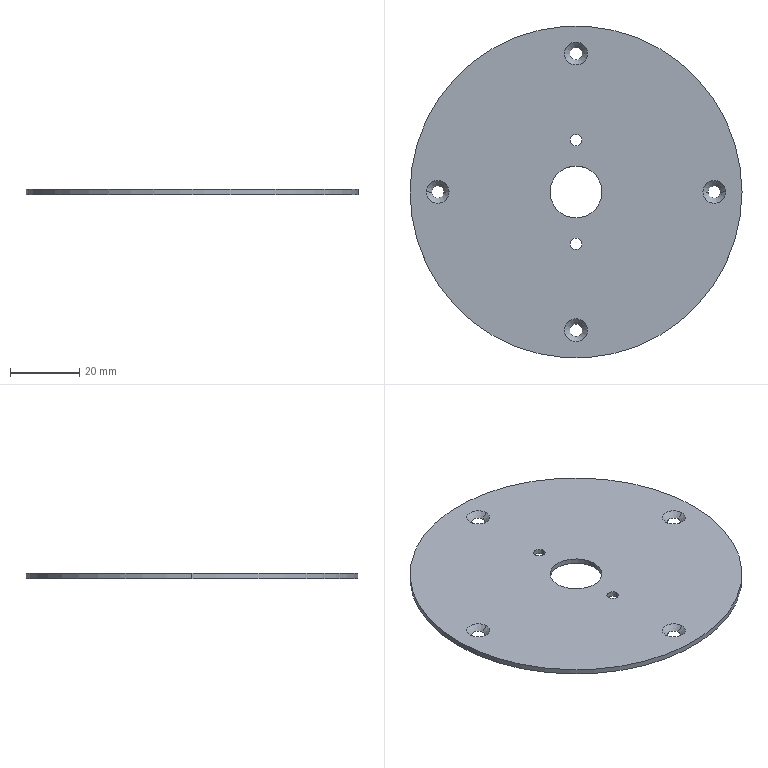Part | STEP file | Twist motor main pulley clamp plate SGN-4-10 | 1 solid | 18 faces | box 96 x 96 x 1.5 mm | volume 10441 mm3 | cylinder 8 | cone 8 | plane 2 | commonest cylinder face diameters 3.3 x4 15 x2 96 x2
STEP:
#1=CARTESIAN_POINT('',(0.,0.,0.));
#2=DIRECTION('',(0.,0.,1.));
#3=DIRECTION('',(1.,0.,0.));
#4=AXIS2_PLACEMENT_3D('',#1,#2,#3);
#5=CARTESIAN_POINT('',(1.65,15.,-1.5));
#6=VERTEX_POINT('',#5);
#7=CARTESIAN_POINT('',(1.65,15.,0.));
#8=VERTEX_POINT('',#7);
#9=CARTESIAN_POINT('',(1.65,15.,0.));
#10=DIRECTION('',(0.,0.,1.));
#11=VECTOR('',#10,1.);
#12=LINE('',#9,#11);
#13=CARTESIAN_POINT('',(0.,15.,0.));
#14=DIRECTION('',(0.,0.,1.));
#15=DIRECTION('',(1.,0.,0.));
#16=AXIS2_PLACEMENT_3D('',#13,#14,#15);
#17=CYLINDRICAL_SURFACE('',#16,1.65);
#18=CARTESIAN_POINT('',(6.283,0.));
#19=DIRECTION('',(0.,1.));
#20=VECTOR('',#19,1.);
#21=LINE('',#18,#20);
#22=(GEOMETRIC_REPRESENTATION_CONTEXT(2)PARAMETRIC_REPRESENTATION_CONTEXT()REPRESENTATION_CONTEXT('',''));
#23=DEFINITIONAL_REPRESENTATION('',(#21),#22);
#24=PCURVE('',#17,#23);
#25=CARTESIAN_POINT('',(0.,15.,0.));
#26=DIRECTION('',(0.,0.,1.));
#27=DIRECTION('',(1.,0.,0.));
#28=AXIS2_PLACEMENT_3D('',#25,#26,#27);
#29=CYLINDRICAL_SURFACE('',#28,1.65);
#30=CARTESIAN_POINT('',(0.,0.));
#31=DIRECTION('',(0.,1.));
#32=VECTOR('',#31,1.);
#33=LINE('',#30,#32);
#34=(GEOMETRIC_REPRESENTATION_CONTEXT(2)PARAMETRIC_REPRESENTATION_CONTEXT()REPRESENTATION_CONTEXT('',''));
#35=DEFINITIONAL_REPRESENTATION('',(#33),#34);
#36=PCURVE('',#29,#35);
#37=SURFACE_CURVE('',#12,(#24,#36),.PCURVE_S1.);
#38=EDGE_CURVE('',#6,#8,#37,.T.);
#39=ORIENTED_EDGE('',*,*,#38,.T.);
#40=CARTESIAN_POINT('',(-1.65,15.,0.));
#41=VERTEX_POINT('',#40);
#42=CARTESIAN_POINT('',(0.,15.,0.));
#43=DIRECTION('',(0.,0.,1.));
#44=DIRECTION('',(1.,0.,0.));
#45=AXIS2_PLACEMENT_3D('',#42,#43,#44);
#46=CIRCLE('',#45,1.65);
#47=CARTESIAN_POINT('',(0.,0.));
#48=DIRECTION('',(1.,0.));
#49=VECTOR('',#48,1.);
#50=LINE('',#47,#49);
#51=(GEOMETRIC_REPRESENTATION_CONTEXT(2)PARAMETRIC_REPRESENTATION_CONTEXT()REPRESENTATION_CONTEXT('',''));
#52=DEFINITIONAL_REPRESENTATION('',(#50),#51);
#53=PCURVE('',#17,#52);
#54=CARTESIAN_POINT('',(0.,0.,0.));
#55=DIRECTION('',(0.,0.,1.));
#56=DIRECTION('',(1.,0.,0.));
#57=AXIS2_PLACEMENT_3D('',#54,#55,#56);
#58=PLANE('',#57);
#59=CARTESIAN_POINT('',(0.,15.));
#60=DIRECTION('',(1.,0.));
#61=AXIS2_PLACEMENT_2D('',#59,#60);
#62=CIRCLE('',#61,1.65);
#63=(GEOMETRIC_REPRESENTATION_CONTEXT(2)PARAMETRIC_REPRESENTATION_CONTEXT()REPRESENTATION_CONTEXT('',''));
#64=DEFINITIONAL_REPRESENTATION('',(#62),#63);
#65=PCURVE('',#58,#64);
#66=SURFACE_CURVE('',#46,(#53,#65),.PCURVE_S1.);
#67=EDGE_CURVE('',#41,#8,#66,.T.);
#68=ORIENTED_EDGE('',*,*,#67,.F.);
#69=CARTESIAN_POINT('',(-1.65,15.,-1.5));
#70=VERTEX_POINT('',#69);
#71=CARTESIAN_POINT('',(-1.65,15.,0.));
#72=DIRECTION('',(0.,0.,1.));
#73=VECTOR('',#72,1.);
#74=LINE('',#71,#73);
#75=CARTESIAN_POINT('',(3.142,0.));
#76=DIRECTION('',(0.,1.));
#77=VECTOR('',#76,1.);
#78=LINE('',#75,#77);
#79=(GEOMETRIC_REPRESENTATION_CONTEXT(2)PARAMETRIC_REPRESENTATION_CONTEXT()REPRESENTATION_CONTEXT('',''));
#80=DEFINITIONAL_REPRESENTATION('',(#78),#79);
#81=PCURVE('',#17,#80);
#82=CARTESIAN_POINT('',(3.142,0.));
#83=DIRECTION('',(0.,1.));
#84=VECTOR('',#83,1.);
#85=LINE('',#82,#84);
#86=(GEOMETRIC_REPRESENTATION_CONTEXT(2)PARAMETRIC_REPRESENTATION_CONTEXT()REPRESENTATION_CONTEXT('',''));
#87=DEFINITIONAL_REPRESENTATION('',(#85),#86);
#88=PCURVE('',#29,#87);
#89=SURFACE_CURVE('',#74,(#81,#88),.PCURVE_S1.);
#90=EDGE_CURVE('',#70,#41,#89,.T.);
#91=ORIENTED_EDGE('',*,*,#90,.F.);
#92=CARTESIAN_POINT('',(0.,15.,-1.5));
#93=DIRECTION('',(0.,0.,1.));
#94=DIRECTION('',(1.,0.,0.));
#95=AXIS2_PLACEMENT_3D('',#92,#93,#94);
#96=CIRCLE('',#95,1.65);
#97=CARTESIAN_POINT('',(0.,-1.5));
#98=DIRECTION('',(1.,0.));
#99=VECTOR('',#98,1.);
#100=LINE('',#97,#99);
#101=(GEOMETRIC_REPRESENTATION_CONTEXT(2)PARAMETRIC_REPRESENTATION_CONTEXT()REPRESENTATION_CONTEXT('',''));
#102=DEFINITIONAL_REPRESENTATION('',(#100),#101);
#103=PCURVE('',#17,#102);
#104=CARTESIAN_POINT('',(0.,0.,-1.5));
#105=DIRECTION('',(0.,0.,1.));
#106=DIRECTION('',(1.,0.,0.));
#107=AXIS2_PLACEMENT_3D('',#104,#105,#106);
#108=PLANE('',#107);
#109=CARTESIAN_POINT('',(0.,15.));
#110=DIRECTION('',(1.,0.));
#111=AXIS2_PLACEMENT_2D('',#109,#110);
#112=CIRCLE('',#111,1.65);
#113=(GEOMETRIC_REPRESENTATION_CONTEXT(2)PARAMETRIC_REPRESENTATION_CONTEXT()REPRESENTATION_CONTEXT('',''));
#114=DEFINITIONAL_REPRESENTATION('',(#112),#113);
#115=PCURVE('',#108,#114);
#116=SURFACE_CURVE('',#96,(#103,#115),.PCURVE_S1.);
#117=EDGE_CURVE('',#70,#6,#116,.T.);
#118=ORIENTED_EDGE('',*,*,#117,.T.);
#119=EDGE_LOOP('',(#39,#68,#91,#118));
#120=FACE_BOUND('',#119,.F.);
#121=ADVANCED_FACE('',(#120),#17,.F.);
#122=CARTESIAN_POINT('',(1.65,-15.,-1.5));
#123=VERTEX_POINT('',#122);
#124=CARTESIAN_POINT('',(1.65,-15.,0.));
#125=VERTEX_POINT('',#124);
#126=CARTESIAN_POINT('',(1.65,-15.,0.));
#127=DIRECTION('',(0.,0.,1.));
#128=VECTOR('',#127,1.);
#129=LINE('',#126,#128);
#130=CARTESIAN_POINT('',(0.,-15.,0.));
#131=DIRECTION('',(0.,0.,1.));
#132=DIRECTION('',(1.,0.,0.));
#133=AXIS2_PLACEMENT_3D('',#130,#131,#132);
#134=CYLINDRICAL_SURFACE('',#133,1.65);
#135=CARTESIAN_POINT('',(6.283,0.));
#136=DIRECTION('',(0.,1.));
#137=VECTOR('',#136,1.);
#138=LINE('',#135,#137);
#139=(GEOMETRIC_REPRESENTATION_CONTEXT(2)PARAMETRIC_REPRESENTATION_CONTEXT()REPRESENTATION_CONTEXT('',''));
#140=DEFINITIONAL_REPRESENTATION('',(#138),#139);
#141=PCURVE('',#134,#140);
#142=CARTESIAN_POINT('',(0.,-15.,0.));
#143=DIRECTION('',(0.,0.,1.));
#144=DIRECTION('',(1.,0.,0.));
#145=AXIS2_PLACEMENT_3D('',#142,#143,#144);
#146=CYLINDRICAL_SURFACE('',#145,1.65);
#147=CARTESIAN_POINT('',(0.,0.));
#148=DIRECTION('',(0.,1.));
#149=VECTOR('',#148,1.);
#150=LINE('',#147,#149);
#151=(GEOMETRIC_REPRESENTATION_CONTEXT(2)PARAMETRIC_REPRESENTATION_CONTEXT()REPRESENTATION_CONTEXT('',''));
#152=DEFINITIONAL_REPRESENTATION('',(#150),#151);
#153=PCURVE('',#146,#152);
#154=SURFACE_CURVE('',#129,(#141,#153),.PCURVE_S1.);
#155=EDGE_CURVE('',#123,#125,#154,.T.);
#156=ORIENTED_EDGE('',*,*,#155,.T.);
#157=CARTESIAN_POINT('',(-1.65,-15.,0.));
#158=VERTEX_POINT('',#157);
#159=CARTESIAN_POINT('',(0.,-15.,0.));
#160=DIRECTION('',(0.,0.,1.));
#161=DIRECTION('',(1.,0.,0.));
#162=AXIS2_PLACEMENT_3D('',#159,#160,#161);
#163=CIRCLE('',#162,1.65);
#164=CARTESIAN_POINT('',(0.,0.));
#165=DIRECTION('',(1.,0.));
#166=VECTOR('',#165,1.);
#167=LINE('',#164,#166);
#168=(GEOMETRIC_REPRESENTATION_CONTEXT(2)PARAMETRIC_REPRESENTATION_CONTEXT()REPRESENTATION_CONTEXT('',''));
#169=DEFINITIONAL_REPRESENTATION('',(#167),#168);
#170=PCURVE('',#134,#169);
#171=CARTESIAN_POINT('',(0.,-15.));
#172=DIRECTION('',(1.,0.));
#173=AXIS2_PLACEMENT_2D('',#171,#172);
#174=CIRCLE('',#173,1.65);
#175=(GEOMETRIC_REPRESENTATION_CONTEXT(2)PARAMETRIC_REPRESENTATION_CONTEXT()REPRESENTATION_CONTEXT('',''));
#176=DEFINITIONAL_REPRESENTATION('',(#174),#175);
#177=PCURVE('',#58,#176);
#178=SURFACE_CURVE('',#163,(#170,#177),.PCURVE_S1.);
#179=EDGE_CURVE('',#158,#125,#178,.T.);
#180=ORIENTED_EDGE('',*,*,#179,.F.);
#181=CARTESIAN_POINT('',(-1.65,-15.,-1.5));
#182=VERTEX_POINT('',#181);
#183=CARTESIAN_POINT('',(-1.65,-15.,0.));
#184=DIRECTION('',(0.,0.,1.));
#185=VECTOR('',#184,1.);
#186=LINE('',#183,#185);
#187=CARTESIAN_POINT('',(3.142,0.));
#188=DIRECTION('',(0.,1.));
#189=VECTOR('',#188,1.);
#190=LINE('',#187,#189);
#191=(GEOMETRIC_REPRESENTATION_CONTEXT(2)PARAMETRIC_REPRESENTATION_CONTEXT()REPRESENTATION_CONTEXT('',''));
#192=DEFINITIONAL_REPRESENTATION('',(#190),#191);
#193=PCURVE('',#134,#192);
#194=CARTESIAN_POINT('',(3.142,0.));
#195=DIRECTION('',(0.,1.));
#196=VECTOR('',#195,1.);
#197=LINE('',#194,#196);
#198=(GEOMETRIC_REPRESENTATION_CONTEXT(2)PARAMETRIC_REPRESENTATION_CONTEXT()REPRESENTATION_CONTEXT('',''));
#199=DEFINITIONAL_REPRESENTATION('',(#197),#198);
#200=PCURVE('',#146,#199);
#201=SURFACE_CURVE('',#186,(#193,#200),.PCURVE_S1.);
#202=EDGE_CURVE('',#182,#158,#201,.T.);
#203=ORIENTED_EDGE('',*,*,#202,.F.);
#204=CARTESIAN_POINT('',(0.,-15.,-1.5));
#205=DIRECTION('',(0.,0.,1.));
#206=DIRECTION('',(1.,0.,0.));
#207=AXIS2_PLACEMENT_3D('',#204,#205,#206);
#208=CIRCLE('',#207,1.65);
#209=CARTESIAN_POINT('',(0.,-1.5));
#210=DIRECTION('',(1.,0.));
#211=VECTOR('',#210,1.);
#212=LINE('',#209,#211);
#213=(GEOMETRIC_REPRESENTATION_CONTEXT(2)PARAMETRIC_REPRESENTATION_CONTEXT()REPRESENTATION_CONTEXT('',''));
#214=DEFINITIONAL_REPRESENTATION('',(#212),#213);
#215=PCURVE('',#134,#214);
#216=CARTESIAN_POINT('',(0.,-15.));
#217=DIRECTION('',(1.,0.));
#218=AXIS2_PLACEMENT_2D('',#216,#217);
#219=CIRCLE('',#218,1.65);
#220=(GEOMETRIC_REPRESENTATION_CONTEXT(2)PARAMETRIC_REPRESENTATION_CONTEXT()REPRESENTATION_CONTEXT('',''));
#221=DEFINITIONAL_REPRESENTATION('',(#219),#220);
#222=PCURVE('',#108,#221);
#223=SURFACE_CURVE('',#208,(#215,#222),.PCURVE_S1.);
#224=EDGE_CURVE('',#182,#123,#223,.T.);
#225=ORIENTED_EDGE('',*,*,#224,.T.);
#226=EDGE_LOOP('',(#156,#180,#203,#225));
#227=FACE_BOUND('',#226,.F.);
#228=ADVANCED_FACE('',(#227),#134,.F.);
#229=CARTESIAN_POINT('',(7.5,0.,-1.5));
#230=VERTEX_POINT('',#229);
#231=CARTESIAN_POINT('',(7.5,0.,0.));
#232=VERTEX_POINT('',#231);
#233=CARTESIAN_POINT('',(7.5,0.,-10.));
#234=DIRECTION('',(0.,0.,1.));
#235=VECTOR('',#234,1.);
#236=LINE('',#233,#235);
#237=CARTESIAN_POINT('',(0.,0.,-10.));
#238=DIRECTION('',(0.,0.,1.));
#239=DIRECTION('',(1.,0.,0.));
#240=AXIS2_PLACEMENT_3D('',#237,#238,#239);
#241=CYLINDRICAL_SURFACE('',#240,7.5);
#242=CARTESIAN_POINT('',(6.283,0.));
#243=DIRECTION('',(0.,1.));
#244=VECTOR('',#243,1.);
#245=LINE('',#242,#244);
#246=(GEOMETRIC_REPRESENTATION_CONTEXT(2)PARAMETRIC_REPRESENTATION_CONTEXT()REPRESENTATION_CONTEXT('',''));
#247=DEFINITIONAL_REPRESENTATION('',(#245),#246);
#248=PCURVE('',#241,#247);
#249=CARTESIAN_POINT('',(0.,0.,-10.));
#250=DIRECTION('',(0.,0.,1.));
#251=DIRECTION('',(1.,0.,0.));
#252=AXIS2_PLACEMENT_3D('',#249,#250,#251);
#253=CYLINDRICAL_SURFACE('',#252,7.5);
#254=CARTESIAN_POINT('',(0.,0.));
#255=DIRECTION('',(0.,1.));
#256=VECTOR('',#255,1.);
#257=LINE('',#254,#256);
#258=(GEOMETRIC_REPRESENTATION_CONTEXT(2)PARAMETRIC_REPRESENTATION_CONTEXT()REPRESENTATION_CONTEXT('',''));
#259=DEFINITIONAL_REPRESENTATION('',(#257),#258);
#260=PCURVE('',#253,#259);
#261=SURFACE_CURVE('',#236,(#248,#260),.PCURVE_S1.);
#262=EDGE_CURVE('',#230,#232,#261,.T.);
#263=ORIENTED_EDGE('',*,*,#262,.T.);
#264=CARTESIAN_POINT('',(-7.5,0.,0.));
#265=VERTEX_POINT('',#264);
#266=CARTESIAN_POINT('',(0.,0.,0.));
#267=DIRECTION('',(0.,0.,1.));
#268=DIRECTION('',(1.,0.,0.));
#269=AXIS2_PLACEMENT_3D('',#266,#267,#268);
#270=CIRCLE('',#269,7.5);
#271=CARTESIAN_POINT('',(0.,10.));
#272=DIRECTION('',(1.,0.));
#273=VECTOR('',#272,1.);
#274=LINE('',#271,#273);
#275=(GEOMETRIC_REPRESENTATION_CONTEXT(2)PARAMETRIC_REPRESENTATION_CONTEXT()REPRESENTATION_CONTEXT('',''));
#276=DEFINITIONAL_REPRESENTATION('',(#274),#275);
#277=PCURVE('',#241,#276);
#278=CARTESIAN_POINT('',(0.,0.));
#279=DIRECTION('',(1.,0.));
#280=AXIS2_PLACEMENT_2D('',#278,#279);
#281=CIRCLE('',#280,7.5);
#282=(GEOMETRIC_REPRESENTATION_CONTEXT(2)PARAMETRIC_REPRESENTATION_CONTEXT()REPRESENTATION_CONTEXT('',''));
#283=DEFINITIONAL_REPRESENTATION('',(#281),#282);
#284=PCURVE('',#58,#283);
#285=SURFACE_CURVE('',#270,(#277,#284),.PCURVE_S1.);
#286=EDGE_CURVE('',#265,#232,#285,.T.);
#287=ORIENTED_EDGE('',*,*,#286,.F.);
#288=CARTESIAN_POINT('',(-7.5,0.,-1.5));
#289=VERTEX_POINT('',#288);
#290=CARTESIAN_POINT('',(-7.5,0.,-10.));
#291=DIRECTION('',(0.,0.,1.));
#292=VECTOR('',#291,1.);
#293=LINE('',#290,#292);
#294=CARTESIAN_POINT('',(3.142,0.));
#295=DIRECTION('',(0.,1.));
#296=VECTOR('',#295,1.);
#297=LINE('',#294,#296);
#298=(GEOMETRIC_REPRESENTATION_CONTEXT(2)PARAMETRIC_REPRESENTATION_CONTEXT()REPRESENTATION_CONTEXT('',''));
#299=DEFINITIONAL_REPRESENTATION('',(#297),#298);
#300=PCURVE('',#241,#299);
#301=CARTESIAN_POINT('',(3.142,0.));
#302=DIRECTION('',(0.,1.));
#303=VECTOR('',#302,1.);
#304=LINE('',#301,#303);
#305=(GEOMETRIC_REPRESENTATION_CONTEXT(2)PARAMETRIC_REPRESENTATION_CONTEXT()REPRESENTATION_CONTEXT('',''));
#306=DEFINITIONAL_REPRESENTATION('',(#304),#305);
#307=PCURVE('',#253,#306);
#308=SURFACE_CURVE('',#293,(#300,#307),.PCURVE_S1.);
#309=EDGE_CURVE('',#289,#265,#308,.T.);
#310=ORIENTED_EDGE('',*,*,#309,.F.);
#311=CARTESIAN_POINT('',(0.,0.,-1.5));
#312=DIRECTION('',(0.,0.,1.));
#313=DIRECTION('',(1.,0.,0.));
#314=AXIS2_PLACEMENT_3D('',#311,#312,#313);
#315=CIRCLE('',#314,7.5);
#316=CARTESIAN_POINT('',(0.,8.5));
#317=DIRECTION('',(1.,0.));
#318=VECTOR('',#317,1.);
#319=LINE('',#316,#318);
#320=(GEOMETRIC_REPRESENTATION_CONTEXT(2)PARAMETRIC_REPRESENTATION_CONTEXT()REPRESENTATION_CONTEXT('',''));
#321=DEFINITIONAL_REPRESENTATION('',(#319),#320);
#322=PCURVE('',#241,#321);
#323=CARTESIAN_POINT('',(0.,0.));
#324=DIRECTION('',(1.,0.));
#325=AXIS2_PLACEMENT_2D('',#323,#324);
#326=CIRCLE('',#325,7.5);
#327=(GEOMETRIC_REPRESENTATION_CONTEXT(2)PARAMETRIC_REPRESENTATION_CONTEXT()REPRESENTATION_CONTEXT('',''));
#328=DEFINITIONAL_REPRESENTATION('',(#326),#327);
#329=PCURVE('',#108,#328);
#330=SURFACE_CURVE('',#315,(#322,#329),.PCURVE_S1.);
#331=EDGE_CURVE('',#289,#230,#330,.T.);
#332=ORIENTED_EDGE('',*,*,#331,.T.);
#333=EDGE_LOOP('',(#263,#287,#310,#332));
#334=FACE_BOUND('',#333,.F.);
#335=ADVANCED_FACE('',(#334),#241,.F.);
#336=CARTESIAN_POINT('',(1.8,40.,-1.5));
#337=VERTEX_POINT('',#336);
#338=CARTESIAN_POINT('',(3.3,40.,0.));
#339=VERTEX_POINT('',#338);
#340=CARTESIAN_POINT('',(3.3,40.,0.));
#341=DIRECTION('',(0.7071,0.,0.7071));
#342=VECTOR('',#341,1.);
#343=LINE('',#340,#342);
#344=CARTESIAN_POINT('',(0.,40.,0.));
#345=DIRECTION('',(0.,0.,1.));
#346=DIRECTION('',(1.,0.,0.));
#347=AXIS2_PLACEMENT_3D('',#344,#345,#346);
#348=CONICAL_SURFACE('',#347,3.3,0.7854);
#349=CARTESIAN_POINT('',(6.283,0.));
#350=DIRECTION('',(0.,1.));
#351=VECTOR('',#350,1.);
#352=LINE('',#349,#351);
#353=(GEOMETRIC_REPRESENTATION_CONTEXT(2)PARAMETRIC_REPRESENTATION_CONTEXT()REPRESENTATION_CONTEXT('',''));
#354=DEFINITIONAL_REPRESENTATION('',(#352),#353);
#355=PCURVE('',#348,#354);
#356=CARTESIAN_POINT('',(0.,40.,0.));
#357=DIRECTION('',(0.,0.,1.));
#358=DIRECTION('',(1.,0.,0.));
#359=AXIS2_PLACEMENT_3D('',#356,#357,#358);
#360=CONICAL_SURFACE('',#359,3.3,0.7854);
#361=CARTESIAN_POINT('',(0.,0.));
#362=DIRECTION('',(0.,1.));
#363=VECTOR('',#362,1.);
#364=LINE('',#361,#363);
#365=(GEOMETRIC_REPRESENTATION_CONTEXT(2)PARAMETRIC_REPRESENTATION_CONTEXT()REPRESENTATION_CONTEXT('',''));
#366=DEFINITIONAL_REPRESENTATION('',(#364),#365);
#367=PCURVE('',#360,#366);
#368=SURFACE_CURVE('',#343,(#355,#367),.PCURVE_S1.);
#369=EDGE_CURVE('',#337,#339,#368,.T.);
#370=ORIENTED_EDGE('',*,*,#369,.T.);
#371=CARTESIAN_POINT('',(-3.3,40.,0.));
#372=VERTEX_POINT('',#371);
#373=CARTESIAN_POINT('',(0.,40.,0.));
#374=DIRECTION('',(0.,0.,1.));
#375=DIRECTION('',(1.,0.,0.));
#376=AXIS2_PLACEMENT_3D('',#373,#374,#375);
#377=CIRCLE('',#376,3.3);
#378=CARTESIAN_POINT('',(0.,0.));
#379=DIRECTION('',(1.,0.));
#380=VECTOR('',#379,1.);
#381=LINE('',#378,#380);
#382=(GEOMETRIC_REPRESENTATION_CONTEXT(2)PARAMETRIC_REPRESENTATION_CONTEXT()REPRESENTATION_CONTEXT('',''));
#383=DEFINITIONAL_REPRESENTATION('',(#381),#382);
#384=PCURVE('',#348,#383);
#385=CARTESIAN_POINT('',(0.,40.));
#386=DIRECTION('',(1.,0.));
#387=AXIS2_PLACEMENT_2D('',#385,#386);
#388=CIRCLE('',#387,3.3);
#389=(GEOMETRIC_REPRESENTATION_CONTEXT(2)PARAMETRIC_REPRESENTATION_CONTEXT()REPRESENTATION_CONTEXT('',''));
#390=DEFINITIONAL_REPRESENTATION('',(#388),#389);
#391=PCURVE('',#58,#390);
#392=SURFACE_CURVE('',#377,(#384,#391),.PCURVE_S1.);
#393=EDGE_CURVE('',#372,#339,#392,.T.);
#394=ORIENTED_EDGE('',*,*,#393,.F.);
#395=CARTESIAN_POINT('',(-1.8,40.,-1.5));
#396=VERTEX_POINT('',#395);
#397=CARTESIAN_POINT('',(-3.3,40.,0.));
#398=DIRECTION('',(-0.7071,0.,0.7071));
#399=VECTOR('',#398,1.);
#400=LINE('',#397,#399);
#401=CARTESIAN_POINT('',(3.142,0.));
#402=DIRECTION('',(0.,1.));
#403=VECTOR('',#402,1.);
#404=LINE('',#401,#403);
#405=(GEOMETRIC_REPRESENTATION_CONTEXT(2)PARAMETRIC_REPRESENTATION_CONTEXT()REPRESENTATION_CONTEXT('',''));
#406=DEFINITIONAL_REPRESENTATION('',(#404),#405);
#407=PCURVE('',#348,#406);
#408=CARTESIAN_POINT('',(3.142,0.));
#409=DIRECTION('',(0.,1.));
#410=VECTOR('',#409,1.);
#411=LINE('',#408,#410);
#412=(GEOMETRIC_REPRESENTATION_CONTEXT(2)PARAMETRIC_REPRESENTATION_CONTEXT()REPRESENTATION_CONTEXT('',''));
#413=DEFINITIONAL_REPRESENTATION('',(#411),#412);
#414=PCURVE('',#360,#413);
#415=SURFACE_CURVE('',#400,(#407,#414),.PCURVE_S1.);
#416=EDGE_CURVE('',#396,#372,#415,.T.);
#417=ORIENTED_EDGE('',*,*,#416,.F.);
#418=CARTESIAN_POINT('',(0.,40.,-1.5));
#419=DIRECTION('',(0.,0.,1.));
#420=DIRECTION('',(1.,0.,0.));
#421=AXIS2_PLACEMENT_3D('',#418,#419,#420);
#422=CIRCLE('',#421,1.8);
#423=CARTESIAN_POINT('',(0.,-1.5));
#424=DIRECTION('',(1.,0.));
#425=VECTOR('',#424,1.);
#426=LINE('',#423,#425);
#427=(GEOMETRIC_REPRESENTATION_CONTEXT(2)PARAMETRIC_REPRESENTATION_CONTEXT()REPRESENTATION_CONTEXT('',''));
#428=DEFINITIONAL_REPRESENTATION('',(#426),#427);
#429=PCURVE('',#348,#428);
#430=CARTESIAN_POINT('',(0.,40.));
#431=DIRECTION('',(1.,0.));
#432=AXIS2_PLACEMENT_2D('',#430,#431);
#433=CIRCLE('',#432,1.8);
#434=(GEOMETRIC_REPRESENTATION_CONTEXT(2)PARAMETRIC_REPRESENTATION_CONTEXT()REPRESENTATION_CONTEXT('',''));
#435=DEFINITIONAL_REPRESENTATION('',(#433),#434);
#436=PCURVE('',#108,#435);
#437=SURFACE_CURVE('',#422,(#429,#436),.PCURVE_S1.);
#438=EDGE_CURVE('',#396,#337,#437,.T.);
#439=ORIENTED_EDGE('',*,*,#438,.T.);
#440=EDGE_LOOP('',(#370,#394,#417,#439));
#441=FACE_BOUND('',#440,.F.);
#442=ADVANCED_FACE('',(#441),#348,.F.);
#443=CARTESIAN_POINT('',(41.8,0.,-1.5));
#444=VERTEX_POINT('',#443);
#445=CARTESIAN_POINT('',(43.3,0.,0.));
#446=VERTEX_POINT('',#445);
#447=CARTESIAN_POINT('',(43.3,0.,0.));
#448=DIRECTION('',(0.7071,0.,0.7071));
#449=VECTOR('',#448,1.);
#450=LINE('',#447,#449);
#451=CARTESIAN_POINT('',(40.,0.,0.));
#452=DIRECTION('',(0.,0.,1.));
#453=DIRECTION('',(1.,0.,0.));
#454=AXIS2_PLACEMENT_3D('',#451,#452,#453);
#455=CONICAL_SURFACE('',#454,3.3,0.7854);
#456=CARTESIAN_POINT('',(6.283,0.));
#457=DIRECTION('',(0.,1.));
#458=VECTOR('',#457,1.);
#459=LINE('',#456,#458);
#460=(GEOMETRIC_REPRESENTATION_CONTEXT(2)PARAMETRIC_REPRESENTATION_CONTEXT()REPRESENTATION_CONTEXT('',''));
#461=DEFINITIONAL_REPRESENTATION('',(#459),#460);
#462=PCURVE('',#455,#461);
#463=CARTESIAN_POINT('',(40.,0.,0.));
#464=DIRECTION('',(0.,0.,1.));
#465=DIRECTION('',(1.,0.,0.));
#466=AXIS2_PLACEMENT_3D('',#463,#464,#465);
#467=CONICAL_SURFACE('',#466,3.3,0.7854);
#468=CARTESIAN_POINT('',(0.,0.));
#469=DIRECTION('',(0.,1.));
#470=VECTOR('',#469,1.);
#471=LINE('',#468,#470);
#472=(GEOMETRIC_REPRESENTATION_CONTEXT(2)PARAMETRIC_REPRESENTATION_CONTEXT()REPRESENTATION_CONTEXT('',''));
#473=DEFINITIONAL_REPRESENTATION('',(#471),#472);
#474=PCURVE('',#467,#473);
#475=SURFACE_CURVE('',#450,(#462,#474),.PCURVE_S1.);
#476=EDGE_CURVE('',#444,#446,#475,.T.);
#477=ORIENTED_EDGE('',*,*,#476,.T.);
#478=CARTESIAN_POINT('',(36.7,0.,0.));
#479=VERTEX_POINT('',#478);
#480=CARTESIAN_POINT('',(40.,0.,0.));
#481=DIRECTION('',(0.,0.,1.));
#482=DIRECTION('',(1.,0.,0.));
#483=AXIS2_PLACEMENT_3D('',#480,#481,#482);
#484=CIRCLE('',#483,3.3);
#485=CARTESIAN_POINT('',(0.,0.));
#486=DIRECTION('',(1.,0.));
#487=VECTOR('',#486,1.);
#488=LINE('',#485,#487);
#489=(GEOMETRIC_REPRESENTATION_CONTEXT(2)PARAMETRIC_REPRESENTATION_CONTEXT()REPRESENTATION_CONTEXT('',''));
#490=DEFINITIONAL_REPRESENTATION('',(#488),#489);
#491=PCURVE('',#455,#490);
#492=CARTESIAN_POINT('',(40.,0.));
#493=DIRECTION('',(1.,0.));
#494=AXIS2_PLACEMENT_2D('',#492,#493);
#495=CIRCLE('',#494,3.3);
#496=(GEOMETRIC_REPRESENTATION_CONTEXT(2)PARAMETRIC_REPRESENTATION_CONTEXT()REPRESENTATION_CONTEXT('',''));
#497=DEFINITIONAL_REPRESENTATION('',(#495),#496);
#498=PCURVE('',#58,#497);
#499=SURFACE_CURVE('',#484,(#491,#498),.PCURVE_S1.);
#500=EDGE_CURVE('',#479,#446,#499,.T.);
#501=ORIENTED_EDGE('',*,*,#500,.F.);
#502=CARTESIAN_POINT('',(38.2,0.,-1.5));
#503=VERTEX_POINT('',#502);
#504=CARTESIAN_POINT('',(36.7,0.,0.));
#505=DIRECTION('',(-0.7071,0.,0.7071));
#506=VECTOR('',#505,1.);
#507=LINE('',#504,#506);
#508=CARTESIAN_POINT('',(3.142,0.));
#509=DIRECTION('',(0.,1.));
#510=VECTOR('',#509,1.);
#511=LINE('',#508,#510);
#512=(GEOMETRIC_REPRESENTATION_CONTEXT(2)PARAMETRIC_REPRESENTATION_CONTEXT()REPRESENTATION_CONTEXT('',''));
#513=DEFINITIONAL_REPRESENTATION('',(#511),#512);
#514=PCURVE('',#455,#513);
#515=CARTESIAN_POINT('',(3.142,0.));
#516=DIRECTION('',(0.,1.));
#517=VECTOR('',#516,1.);
#518=LINE('',#515,#517);
#519=(GEOMETRIC_REPRESENTATION_CONTEXT(2)PARAMETRIC_REPRESENTATION_CONTEXT()REPRESENTATION_CONTEXT('',''));
#520=DEFINITIONAL_REPRESENTATION('',(#518),#519);
#521=PCURVE('',#467,#520);
#522=SURFACE_CURVE('',#507,(#514,#521),.PCURVE_S1.);
#523=EDGE_CURVE('',#503,#479,#522,.T.);
#524=ORIENTED_EDGE('',*,*,#523,.F.);
#525=CARTESIAN_POINT('',(40.,0.,-1.5));
#526=DIRECTION('',(0.,0.,1.));
#527=DIRECTION('',(1.,0.,0.));
#528=AXIS2_PLACEMENT_3D('',#525,#526,#527);
#529=CIRCLE('',#528,1.8);
#530=CARTESIAN_POINT('',(0.,-1.5));
#531=DIRECTION('',(1.,0.));
#532=VECTOR('',#531,1.);
#533=LINE('',#530,#532);
#534=(GEOMETRIC_REPRESENTATION_CONTEXT(2)PARAMETRIC_REPRESENTATION_CONTEXT()REPRESENTATION_CONTEXT('',''));
#535=DEFINITIONAL_REPRESENTATION('',(#533),#534);
#536=PCURVE('',#455,#535);
#537=CARTESIAN_POINT('',(40.,0.));
#538=DIRECTION('',(1.,0.));
#539=AXIS2_PLACEMENT_2D('',#537,#538);
#540=CIRCLE('',#539,1.8);
#541=(GEOMETRIC_REPRESENTATION_CONTEXT(2)PARAMETRIC_REPRESENTATION_CONTEXT()REPRESENTATION_CONTEXT('',''));
#542=DEFINITIONAL_REPRESENTATION('',(#540),#541);
#543=PCURVE('',#108,#542);
#544=SURFACE_CURVE('',#529,(#536,#543),.PCURVE_S1.);
#545=EDGE_CURVE('',#503,#444,#544,.T.);
#546=ORIENTED_EDGE('',*,*,#545,.T.);
#547=EDGE_LOOP('',(#477,#501,#524,#546));
#548=FACE_BOUND('',#547,.F.);
#549=ADVANCED_FACE('',(#548),#455,.F.);
#550=CARTESIAN_POINT('',(1.8,-40.,-1.5));
#551=VERTEX_POINT('',#550);
#552=CARTESIAN_POINT('',(3.3,-40.,0.));
#553=VERTEX_POINT('',#552);
#554=CARTESIAN_POINT('',(3.3,-40.,0.));
#555=DIRECTION('',(0.7071,0.,0.7071));
#556=VECTOR('',#555,1.);
#557=LINE('',#554,#556);
#558=CARTESIAN_POINT('',(0.,-40.,0.));
#559=DIRECTION('',(0.,0.,1.));
#560=DIRECTION('',(1.,0.,0.));
#561=AXIS2_PLACEMENT_3D('',#558,#559,#560);
#562=CONICAL_SURFACE('',#561,3.3,0.7854);
#563=CARTESIAN_POINT('',(6.283,0.));
#564=DIRECTION('',(0.,1.));
#565=VECTOR('',#564,1.);
#566=LINE('',#563,#565);
#567=(GEOMETRIC_REPRESENTATION_CONTEXT(2)PARAMETRIC_REPRESENTATION_CONTEXT()REPRESENTATION_CONTEXT('',''));
#568=DEFINITIONAL_REPRESENTATION('',(#566),#567);
#569=PCURVE('',#562,#568);
#570=CARTESIAN_POINT('',(0.,-40.,0.));
#571=DIRECTION('',(0.,0.,1.));
#572=DIRECTION('',(1.,0.,0.));
#573=AXIS2_PLACEMENT_3D('',#570,#571,#572);
#574=CONICAL_SURFACE('',#573,3.3,0.7854);
#575=CARTESIAN_POINT('',(0.,0.));
#576=DIRECTION('',(0.,1.));
#577=VECTOR('',#576,1.);
#578=LINE('',#575,#577);
#579=(GEOMETRIC_REPRESENTATION_CONTEXT(2)PARAMETRIC_REPRESENTATION_CONTEXT()REPRESENTATION_CONTEXT('',''));
#580=DEFINITIONAL_REPRESENTATION('',(#578),#579);
#581=PCURVE('',#574,#580);
#582=SURFACE_CURVE('',#557,(#569,#581),.PCURVE_S1.);
#583=EDGE_CURVE('',#551,#553,#582,.T.);
#584=ORIENTED_EDGE('',*,*,#583,.T.);
#585=CARTESIAN_POINT('',(-3.3,-40.,0.));
#586=VERTEX_POINT('',#585);
#587=CARTESIAN_POINT('',(0.,-40.,0.));
#588=DIRECTION('',(0.,0.,1.));
#589=DIRECTION('',(1.,0.,0.));
#590=AXIS2_PLACEMENT_3D('',#587,#588,#589);
#591=CIRCLE('',#590,3.3);
#592=CARTESIAN_POINT('',(0.,0.));
#593=DIRECTION('',(1.,0.));
#594=VECTOR('',#593,1.);
#595=LINE('',#592,#594);
#596=(GEOMETRIC_REPRESENTATION_CONTEXT(2)PARAMETRIC_REPRESENTATION_CONTEXT()REPRESENTATION_CONTEXT('',''));
#597=DEFINITIONAL_REPRESENTATION('',(#595),#596);
#598=PCURVE('',#562,#597);
#599=CARTESIAN_POINT('',(0.,-40.));
#600=DIRECTION('',(1.,0.));
#601=AXIS2_PLACEMENT_2D('',#599,#600);
#602=CIRCLE('',#601,3.3);
#603=(GEOMETRIC_REPRESENTATION_CONTEXT(2)PARAMETRIC_REPRESENTATION_CONTEXT()REPRESENTATION_CONTEXT('',''));
#604=DEFINITIONAL_REPRESENTATION('',(#602),#603);
#605=PCURVE('',#58,#604);
#606=SURFACE_CURVE('',#591,(#598,#605),.PCURVE_S1.);
#607=EDGE_CURVE('',#586,#553,#606,.T.);
#608=ORIENTED_EDGE('',*,*,#607,.F.);
#609=CARTESIAN_POINT('',(-1.8,-40.,-1.5));
#610=VERTEX_POINT('',#609);
#611=CARTESIAN_POINT('',(-3.3,-40.,0.));
#612=DIRECTION('',(-0.7071,0.,0.7071));
#613=VECTOR('',#612,1.);
#614=LINE('',#611,#613);
#615=CARTESIAN_POINT('',(3.142,0.));
#616=DIRECTION('',(0.,1.));
#617=VECTOR('',#616,1.);
#618=LINE('',#615,#617);
#619=(GEOMETRIC_REPRESENTATION_CONTEXT(2)PARAMETRIC_REPRESENTATION_CONTEXT()REPRESENTATION_CONTEXT('',''));
#620=DEFINITIONAL_REPRESENTATION('',(#618),#619);
#621=PCURVE('',#562,#620);
#622=CARTESIAN_POINT('',(3.142,0.));
#623=DIRECTION('',(0.,1.));
#624=VECTOR('',#623,1.);
#625=LINE('',#622,#624);
#626=(GEOMETRIC_REPRESENTATION_CONTEXT(2)PARAMETRIC_REPRESENTATION_CONTEXT()REPRESENTATION_CONTEXT('',''));
#627=DEFINITIONAL_REPRESENTATION('',(#625),#626);
#628=PCURVE('',#574,#627);
#629=SURFACE_CURVE('',#614,(#621,#628),.PCURVE_S1.);
#630=EDGE_CURVE('',#610,#586,#629,.T.);
#631=ORIENTED_EDGE('',*,*,#630,.F.);
#632=CARTESIAN_POINT('',(0.,-40.,-1.5));
#633=DIRECTION('',(0.,0.,1.));
#634=DIRECTION('',(1.,0.,0.));
#635=AXIS2_PLACEMENT_3D('',#632,#633,#634);
#636=CIRCLE('',#635,1.8);
#637=CARTESIAN_POINT('',(0.,-1.5));
#638=DIRECTION('',(1.,0.));
#639=VECTOR('',#638,1.);
#640=LINE('',#637,#639);
#641=(GEOMETRIC_REPRESENTATION_CONTEXT(2)PARAMETRIC_REPRESENTATION_CONTEXT()REPRESENTATION_CONTEXT('',''));
#642=DEFINITIONAL_REPRESENTATION('',(#640),#641);
#643=PCURVE('',#562,#642);
#644=CARTESIAN_POINT('',(0.,-40.));
#645=DIRECTION('',(1.,0.));
#646=AXIS2_PLACEMENT_2D('',#644,#645);
#647=CIRCLE('',#646,1.8);
#648=(GEOMETRIC_REPRESENTATION_CONTEXT(2)PARAMETRIC_REPRESENTATION_CONTEXT()REPRESENTATION_CONTEXT('',''));
#649=DEFINITIONAL_REPRESENTATION('',(#647),#648);
#650=PCURVE('',#108,#649);
#651=SURFACE_CURVE('',#636,(#643,#650),.PCURVE_S1.);
#652=EDGE_CURVE('',#610,#551,#651,.T.);
#653=ORIENTED_EDGE('',*,*,#652,.T.);
#654=EDGE_LOOP('',(#584,#608,#631,#653));
#655=FACE_BOUND('',#654,.F.);
#656=ADVANCED_FACE('',(#655),#562,.F.);
#657=CARTESIAN_POINT('',(-38.2,0.,-1.5));
#658=VERTEX_POINT('',#657);
#659=CARTESIAN_POINT('',(-36.7,0.,0.));
#660=VERTEX_POINT('',#659);
#661=CARTESIAN_POINT('',(-36.7,0.,0.));
#662=DIRECTION('',(0.7071,0.,0.7071));
#663=VECTOR('',#662,1.);
#664=LINE('',#661,#663);
#665=CARTESIAN_POINT('',(-40.,0.,0.));
#666=DIRECTION('',(0.,0.,1.));
#667=DIRECTION('',(1.,0.,0.));
#668=AXIS2_PLACEMENT_3D('',#665,#666,#667);
#669=CONICAL_SURFACE('',#668,3.3,0.7854);
#670=CARTESIAN_POINT('',(6.283,0.));
#671=DIRECTION('',(0.,1.));
#672=VECTOR('',#671,1.);
#673=LINE('',#670,#672);
#674=(GEOMETRIC_REPRESENTATION_CONTEXT(2)PARAMETRIC_REPRESENTATION_CONTEXT()REPRESENTATION_CONTEXT('',''));
#675=DEFINITIONAL_REPRESENTATION('',(#673),#674);
#676=PCURVE('',#669,#675);
#677=CARTESIAN_POINT('',(-40.,0.,0.));
#678=DIRECTION('',(0.,0.,1.));
#679=DIRECTION('',(1.,0.,0.));
#680=AXIS2_PLACEMENT_3D('',#677,#678,#679);
#681=CONICAL_SURFACE('',#680,3.3,0.7854);
#682=CARTESIAN_POINT('',(0.,0.));
#683=DIRECTION('',(0.,1.));
#684=VECTOR('',#683,1.);
#685=LINE('',#682,#684);
#686=(GEOMETRIC_REPRESENTATION_CONTEXT(2)PARAMETRIC_REPRESENTATION_CONTEXT()REPRESENTATION_CONTEXT('',''));
#687=DEFINITIONAL_REPRESENTATION('',(#685),#686);
#688=PCURVE('',#681,#687);
#689=SURFACE_CURVE('',#664,(#676,#688),.PCURVE_S1.);
#690=EDGE_CURVE('',#658,#660,#689,.T.);
#691=ORIENTED_EDGE('',*,*,#690,.T.);
#692=CARTESIAN_POINT('',(-43.3,0.,0.));
#693=VERTEX_POINT('',#692);
#694=CARTESIAN_POINT('',(-40.,0.,0.));
#695=DIRECTION('',(0.,0.,1.));
#696=DIRECTION('',(1.,0.,0.));
#697=AXIS2_PLACEMENT_3D('',#694,#695,#696);
#698=CIRCLE('',#697,3.3);
#699=CARTESIAN_POINT('',(0.,0.));
#700=DIRECTION('',(1.,0.));
#701=VECTOR('',#700,1.);
#702=LINE('',#699,#701);
#703=(GEOMETRIC_REPRESENTATION_CONTEXT(2)PARAMETRIC_REPRESENTATION_CONTEXT()REPRESENTATION_CONTEXT('',''));
#704=DEFINITIONAL_REPRESENTATION('',(#702),#703);
#705=PCURVE('',#669,#704);
#706=CARTESIAN_POINT('',(-40.,0.));
#707=DIRECTION('',(1.,0.));
#708=AXIS2_PLACEMENT_2D('',#706,#707);
#709=CIRCLE('',#708,3.3);
#710=(GEOMETRIC_REPRESENTATION_CONTEXT(2)PARAMETRIC_REPRESENTATION_CONTEXT()REPRESENTATION_CONTEXT('',''));
#711=DEFINITIONAL_REPRESENTATION('',(#709),#710);
#712=PCURVE('',#58,#711);
#713=SURFACE_CURVE('',#698,(#705,#712),.PCURVE_S1.);
#714=EDGE_CURVE('',#693,#660,#713,.T.);
#715=ORIENTED_EDGE('',*,*,#714,.F.);
#716=CARTESIAN_POINT('',(-41.8,0.,-1.5));
#717=VERTEX_POINT('',#716);
#718=CARTESIAN_POINT('',(-43.3,0.,0.));
#719=DIRECTION('',(-0.7071,0.,0.7071));
#720=VECTOR('',#719,1.);
#721=LINE('',#718,#720);
#722=CARTESIAN_POINT('',(3.142,0.));
#723=DIRECTION('',(0.,1.));
#724=VECTOR('',#723,1.);
#725=LINE('',#722,#724);
#726=(GEOMETRIC_REPRESENTATION_CONTEXT(2)PARAMETRIC_REPRESENTATION_CONTEXT()REPRESENTATION_CONTEXT('',''));
#727=DEFINITIONAL_REPRESENTATION('',(#725),#726);
#728=PCURVE('',#669,#727);
#729=CARTESIAN_POINT('',(3.142,0.));
#730=DIRECTION('',(0.,1.));
#731=VECTOR('',#730,1.);
#732=LINE('',#729,#731);
#733=(GEOMETRIC_REPRESENTATION_CONTEXT(2)PARAMETRIC_REPRESENTATION_CONTEXT()REPRESENTATION_CONTEXT('',''));
#734=DEFINITIONAL_REPRESENTATION('',(#732),#733);
#735=PCURVE('',#681,#734);
#736=SURFACE_CURVE('',#721,(#728,#735),.PCURVE_S1.);
#737=EDGE_CURVE('',#717,#693,#736,.T.);
#738=ORIENTED_EDGE('',*,*,#737,.F.);
#739=CARTESIAN_POINT('',(-40.,0.,-1.5));
#740=DIRECTION('',(0.,0.,1.));
#741=DIRECTION('',(1.,0.,0.));
#742=AXIS2_PLACEMENT_3D('',#739,#740,#741);
#743=CIRCLE('',#742,1.8);
#744=CARTESIAN_POINT('',(0.,-1.5));
#745=DIRECTION('',(1.,0.));
#746=VECTOR('',#745,1.);
#747=LINE('',#744,#746);
#748=(GEOMETRIC_REPRESENTATION_CONTEXT(2)PARAMETRIC_REPRESENTATION_CONTEXT()REPRESENTATION_CONTEXT('',''));
#749=DEFINITIONAL_REPRESENTATION('',(#747),#748);
#750=PCURVE('',#669,#749);
#751=CARTESIAN_POINT('',(-40.,0.));
#752=DIRECTION('',(1.,0.));
#753=AXIS2_PLACEMENT_2D('',#751,#752);
#754=CIRCLE('',#753,1.8);
#755=(GEOMETRIC_REPRESENTATION_CONTEXT(2)PARAMETRIC_REPRESENTATION_CONTEXT()REPRESENTATION_CONTEXT('',''));
#756=DEFINITIONAL_REPRESENTATION('',(#754),#755);
#757=PCURVE('',#108,#756);
#758=SURFACE_CURVE('',#743,(#750,#757),.PCURVE_S1.);
#759=EDGE_CURVE('',#717,#658,#758,.T.);
#760=ORIENTED_EDGE('',*,*,#759,.T.);
#761=EDGE_LOOP('',(#691,#715,#738,#760));
#762=FACE_BOUND('',#761,.F.);
#763=ADVANCED_FACE('',(#762),#669,.F.);
#764=CARTESIAN_POINT('',(48.,0.,-1.5));
#765=VERTEX_POINT('',#764);
#766=CARTESIAN_POINT('',(-48.,0.,-1.5));
#767=VERTEX_POINT('',#766);
#768=CARTESIAN_POINT('',(0.,0.,-1.5));
#769=DIRECTION('',(0.,0.,1.));
#770=DIRECTION('',(1.,0.,0.));
#771=AXIS2_PLACEMENT_3D('',#768,#769,#770);
#772=CIRCLE('',#771,48.);
#773=CARTESIAN_POINT('',(0.,0.,-1.5));
#774=DIRECTION('',(0.,0.,1.));
#775=DIRECTION('',(1.,0.,0.));
#776=AXIS2_PLACEMENT_3D('',#773,#774,#775);
#777=CYLINDRICAL_SURFACE('',#776,48.);
#778=CARTESIAN_POINT('',(0.,0.));
#779=DIRECTION('',(1.,0.));
#780=VECTOR('',#779,1.);
#781=LINE('',#778,#780);
#782=(GEOMETRIC_REPRESENTATION_CONTEXT(2)PARAMETRIC_REPRESENTATION_CONTEXT()REPRESENTATION_CONTEXT('',''));
#783=DEFINITIONAL_REPRESENTATION('',(#781),#782);
#784=PCURVE('',#777,#783);
#785=CARTESIAN_POINT('',(0.,0.));
#786=DIRECTION('',(1.,0.));
#787=AXIS2_PLACEMENT_2D('',#785,#786);
#788=CIRCLE('',#787,48.);
#789=(GEOMETRIC_REPRESENTATION_CONTEXT(2)PARAMETRIC_REPRESENTATION_CONTEXT()REPRESENTATION_CONTEXT('',''));
#790=DEFINITIONAL_REPRESENTATION('',(#788),#789);
#791=PCURVE('',#108,#790);
#792=SURFACE_CURVE('',#772,(#784,#791),.PCURVE_S1.);
#793=EDGE_CURVE('',#765,#767,#792,.T.);
#794=ORIENTED_EDGE('',*,*,#793,.T.);
#795=CARTESIAN_POINT('',(-48.,0.,0.));
#796=VERTEX_POINT('',#795);
#797=CARTESIAN_POINT('',(-48.,0.,-1.5));
#798=DIRECTION('',(0.,0.,1.));
#799=VECTOR('',#798,1.);
#800=LINE('',#797,#799);
#801=CARTESIAN_POINT('',(3.142,0.));
#802=DIRECTION('',(0.,1.));
#803=VECTOR('',#802,1.);
#804=LINE('',#801,#803);
#805=(GEOMETRIC_REPRESENTATION_CONTEXT(2)PARAMETRIC_REPRESENTATION_CONTEXT()REPRESENTATION_CONTEXT('',''));
#806=DEFINITIONAL_REPRESENTATION('',(#804),#805);
#807=PCURVE('',#777,#806);
#808=CARTESIAN_POINT('',(0.,0.,-1.5));
#809=DIRECTION('',(0.,0.,1.));
#810=DIRECTION('',(1.,0.,0.));
#811=AXIS2_PLACEMENT_3D('',#808,#809,#810);
#812=CYLINDRICAL_SURFACE('',#811,48.);
#813=CARTESIAN_POINT('',(3.142,0.));
#814=DIRECTION('',(0.,1.));
#815=VECTOR('',#814,1.);
#816=LINE('',#813,#815);
#817=(GEOMETRIC_REPRESENTATION_CONTEXT(2)PARAMETRIC_REPRESENTATION_CONTEXT()REPRESENTATION_CONTEXT('',''));
#818=DEFINITIONAL_REPRESENTATION('',(#816),#817);
#819=PCURVE('',#812,#818);
#820=SURFACE_CURVE('',#800,(#807,#819),.PCURVE_S1.);
#821=EDGE_CURVE('',#767,#796,#820,.T.);
#822=ORIENTED_EDGE('',*,*,#821,.T.);
#823=CARTESIAN_POINT('',(48.,0.,0.));
#824=VERTEX_POINT('',#823);
#825=CARTESIAN_POINT('',(0.,0.,0.));
#826=DIRECTION('',(0.,0.,1.));
#827=DIRECTION('',(1.,0.,0.));
#828=AXIS2_PLACEMENT_3D('',#825,#826,#827);
#829=CIRCLE('',#828,48.);
#830=CARTESIAN_POINT('',(0.,1.5));
#831=DIRECTION('',(1.,0.));
#832=VECTOR('',#831,1.);
#833=LINE('',#830,#832);
#834=(GEOMETRIC_REPRESENTATION_CONTEXT(2)PARAMETRIC_REPRESENTATION_CONTEXT()REPRESENTATION_CONTEXT('',''));
#835=DEFINITIONAL_REPRESENTATION('',(#833),#834);
#836=PCURVE('',#777,#835);
#837=CARTESIAN_POINT('',(0.,0.));
#838=DIRECTION('',(1.,0.));
#839=AXIS2_PLACEMENT_2D('',#837,#838);
#840=CIRCLE('',#839,48.);
#841=(GEOMETRIC_REPRESENTATION_CONTEXT(2)PARAMETRIC_REPRESENTATION_CONTEXT()REPRESENTATION_CONTEXT('',''));
#842=DEFINITIONAL_REPRESENTATION('',(#840),#841);
#843=PCURVE('',#58,#842);
#844=SURFACE_CURVE('',#829,(#836,#843),.PCURVE_S1.);
#845=EDGE_CURVE('',#824,#796,#844,.T.);
#846=ORIENTED_EDGE('',*,*,#845,.F.);
#847=CARTESIAN_POINT('',(48.,0.,-1.5));
#848=DIRECTION('',(0.,0.,1.));
#849=VECTOR('',#848,1.);
#850=LINE('',#847,#849);
#851=CARTESIAN_POINT('',(0.,0.));
#852=DIRECTION('',(0.,1.));
#853=VECTOR('',#852,1.);
#854=LINE('',#851,#853);
#855=(GEOMETRIC_REPRESENTATION_CONTEXT(2)PARAMETRIC_REPRESENTATION_CONTEXT()REPRESENTATION_CONTEXT('',''));
#856=DEFINITIONAL_REPRESENTATION('',(#854),#855);
#857=PCURVE('',#777,#856);
#858=CARTESIAN_POINT('',(6.283,0.));
#859=DIRECTION('',(0.,1.));
#860=VECTOR('',#859,1.);
#861=LINE('',#858,#860);
#862=(GEOMETRIC_REPRESENTATION_CONTEXT(2)PARAMETRIC_REPRESENTATION_CONTEXT()REPRESENTATION_CONTEXT('',''));
#863=DEFINITIONAL_REPRESENTATION('',(#861),#862);
#864=PCURVE('',#812,#863);
#865=SURFACE_CURVE('',#850,(#857,#864),.PCURVE_S1.);
#866=EDGE_CURVE('',#765,#824,#865,.T.);
#867=ORIENTED_EDGE('',*,*,#866,.F.);
#868=EDGE_LOOP('',(#794,#822,#846,#867));
#869=FACE_BOUND('',#868,.T.);
#870=ADVANCED_FACE('',(#869),#777,.T.);
#871=ORIENTED_EDGE('',*,*,#821,.F.);
#872=CARTESIAN_POINT('',(0.,0.,-1.5));
#873=DIRECTION('',(0.,0.,1.));
#874=DIRECTION('',(1.,0.,0.));
#875=AXIS2_PLACEMENT_3D('',#872,#873,#874);
#876=CIRCLE('',#875,48.);
#877=CARTESIAN_POINT('',(0.,0.));
#878=DIRECTION('',(1.,0.));
#879=VECTOR('',#878,1.);
#880=LINE('',#877,#879);
#881=(GEOMETRIC_REPRESENTATION_CONTEXT(2)PARAMETRIC_REPRESENTATION_CONTEXT()REPRESENTATION_CONTEXT('',''));
#882=DEFINITIONAL_REPRESENTATION('',(#880),#881);
#883=PCURVE('',#812,#882);
#884=CARTESIAN_POINT('',(0.,0.));
#885=DIRECTION('',(1.,0.));
#886=AXIS2_PLACEMENT_2D('',#884,#885);
#887=CIRCLE('',#886,48.);
#888=(GEOMETRIC_REPRESENTATION_CONTEXT(2)PARAMETRIC_REPRESENTATION_CONTEXT()REPRESENTATION_CONTEXT('',''));
#889=DEFINITIONAL_REPRESENTATION('',(#887),#888);
#890=PCURVE('',#108,#889);
#891=SURFACE_CURVE('',#876,(#883,#890),.PCURVE_S1.);
#892=EDGE_CURVE('',#767,#765,#891,.T.);
#893=ORIENTED_EDGE('',*,*,#892,.T.);
#894=ORIENTED_EDGE('',*,*,#866,.T.);
#895=CARTESIAN_POINT('',(0.,0.,0.));
#896=DIRECTION('',(0.,0.,1.));
#897=DIRECTION('',(1.,0.,0.));
#898=AXIS2_PLACEMENT_3D('',#895,#896,#897);
#899=CIRCLE('',#898,48.);
#900=CARTESIAN_POINT('',(0.,1.5));
#901=DIRECTION('',(1.,0.));
#902=VECTOR('',#901,1.);
#903=LINE('',#900,#902);
#904=(GEOMETRIC_REPRESENTATION_CONTEXT(2)PARAMETRIC_REPRESENTATION_CONTEXT()REPRESENTATION_CONTEXT('',''));
#905=DEFINITIONAL_REPRESENTATION('',(#903),#904);
#906=PCURVE('',#812,#905);
#907=CARTESIAN_POINT('',(0.,0.));
#908=DIRECTION('',(1.,0.));
#909=AXIS2_PLACEMENT_2D('',#907,#908);
#910=CIRCLE('',#909,48.);
#911=(GEOMETRIC_REPRESENTATION_CONTEXT(2)PARAMETRIC_REPRESENTATION_CONTEXT()REPRESENTATION_CONTEXT('',''));
#912=DEFINITIONAL_REPRESENTATION('',(#910),#911);
#913=PCURVE('',#58,#912);
#914=SURFACE_CURVE('',#899,(#906,#913),.PCURVE_S1.);
#915=EDGE_CURVE('',#796,#824,#914,.T.);
#916=ORIENTED_EDGE('',*,*,#915,.F.);
#917=EDGE_LOOP('',(#871,#893,#894,#916));
#918=FACE_BOUND('',#917,.T.);
#919=ADVANCED_FACE('',(#918),#812,.T.);
#920=CARTESIAN_POINT('',(0.,15.,-1.5));
#921=DIRECTION('',(0.,0.,1.));
#922=DIRECTION('',(1.,0.,0.));
#923=AXIS2_PLACEMENT_3D('',#920,#921,#922);
#924=CIRCLE('',#923,1.65);
#925=CARTESIAN_POINT('',(0.,15.));
#926=DIRECTION('',(1.,0.));
#927=AXIS2_PLACEMENT_2D('',#925,#926);
#928=CIRCLE('',#927,1.65);
#929=(GEOMETRIC_REPRESENTATION_CONTEXT(2)PARAMETRIC_REPRESENTATION_CONTEXT()REPRESENTATION_CONTEXT('',''));
#930=DEFINITIONAL_REPRESENTATION('',(#928),#929);
#931=PCURVE('',#108,#930);
#932=CARTESIAN_POINT('',(0.,-1.5));
#933=DIRECTION('',(1.,0.));
#934=VECTOR('',#933,1.);
#935=LINE('',#932,#934);
#936=(GEOMETRIC_REPRESENTATION_CONTEXT(2)PARAMETRIC_REPRESENTATION_CONTEXT()REPRESENTATION_CONTEXT('',''));
#937=DEFINITIONAL_REPRESENTATION('',(#935),#936);
#938=PCURVE('',#29,#937);
#939=SURFACE_CURVE('',#924,(#931,#938),.PCURVE_S1.);
#940=EDGE_CURVE('',#6,#70,#939,.T.);
#941=ORIENTED_EDGE('',*,*,#940,.T.);
#942=ORIENTED_EDGE('',*,*,#117,.T.);
#943=EDGE_LOOP('',(#941,#942));
#944=FACE_BOUND('',#943,.T.);
#945=CARTESIAN_POINT('',(0.,-15.,-1.5));
#946=DIRECTION('',(0.,0.,1.));
#947=DIRECTION('',(1.,0.,0.));
#948=AXIS2_PLACEMENT_3D('',#945,#946,#947);
#949=CIRCLE('',#948,1.65);
#950=CARTESIAN_POINT('',(0.,-15.));
#951=DIRECTION('',(1.,0.));
#952=AXIS2_PLACEMENT_2D('',#950,#951);
#953=CIRCLE('',#952,1.65);
#954=(GEOMETRIC_REPRESENTATION_CONTEXT(2)PARAMETRIC_REPRESENTATION_CONTEXT()REPRESENTATION_CONTEXT('',''));
#955=DEFINITIONAL_REPRESENTATION('',(#953),#954);
#956=PCURVE('',#108,#955);
#957=CARTESIAN_POINT('',(0.,-1.5));
#958=DIRECTION('',(1.,0.));
#959=VECTOR('',#958,1.);
#960=LINE('',#957,#959);
#961=(GEOMETRIC_REPRESENTATION_CONTEXT(2)PARAMETRIC_REPRESENTATION_CONTEXT()REPRESENTATION_CONTEXT('',''));
#962=DEFINITIONAL_REPRESENTATION('',(#960),#961);
#963=PCURVE('',#146,#962);
#964=SURFACE_CURVE('',#949,(#956,#963),.PCURVE_S1.);
#965=EDGE_CURVE('',#123,#182,#964,.T.);
#966=ORIENTED_EDGE('',*,*,#965,.T.);
#967=ORIENTED_EDGE('',*,*,#224,.T.);
#968=EDGE_LOOP('',(#966,#967));
#969=FACE_BOUND('',#968,.T.);
#970=CARTESIAN_POINT('',(0.,0.,-1.5));
#971=DIRECTION('',(0.,0.,1.));
#972=DIRECTION('',(1.,0.,0.));
#973=AXIS2_PLACEMENT_3D('',#970,#971,#972);
#974=CIRCLE('',#973,7.5);
#975=CARTESIAN_POINT('',(0.,0.));
#976=DIRECTION('',(1.,0.));
#977=AXIS2_PLACEMENT_2D('',#975,#976);
#978=CIRCLE('',#977,7.5);
#979=(GEOMETRIC_REPRESENTATION_CONTEXT(2)PARAMETRIC_REPRESENTATION_CONTEXT()REPRESENTATION_CONTEXT('',''));
#980=DEFINITIONAL_REPRESENTATION('',(#978),#979);
#981=PCURVE('',#108,#980);
#982=CARTESIAN_POINT('',(0.,8.5));
#983=DIRECTION('',(1.,0.));
#984=VECTOR('',#983,1.);
#985=LINE('',#982,#984);
#986=(GEOMETRIC_REPRESENTATION_CONTEXT(2)PARAMETRIC_REPRESENTATION_CONTEXT()REPRESENTATION_CONTEXT('',''));
#987=DEFINITIONAL_REPRESENTATION('',(#985),#986);
#988=PCURVE('',#253,#987);
#989=SURFACE_CURVE('',#974,(#981,#988),.PCURVE_S1.);
#990=EDGE_CURVE('',#230,#289,#989,.T.);
#991=ORIENTED_EDGE('',*,*,#990,.T.);
#992=ORIENTED_EDGE('',*,*,#331,.T.);
#993=EDGE_LOOP('',(#991,#992));
#994=FACE_BOUND('',#993,.T.);
#995=CARTESIAN_POINT('',(0.,40.,-1.5));
#996=DIRECTION('',(0.,0.,1.));
#997=DIRECTION('',(1.,0.,0.));
#998=AXIS2_PLACEMENT_3D('',#995,#996,#997);
#999=CIRCLE('',#998,1.8);
#1000=CARTESIAN_POINT('',(0.,40.));
#1001=DIRECTION('',(1.,0.));
#1002=AXIS2_PLACEMENT_2D('',#1000,#1001);
#1003=CIRCLE('',#1002,1.8);
#1004=(GEOMETRIC_REPRESENTATION_CONTEXT(2)PARAMETRIC_REPRESENTATION_CONTEXT()REPRESENTATION_CONTEXT('',''));
#1005=DEFINITIONAL_REPRESENTATION('',(#1003),#1004);
#1006=PCURVE('',#108,#1005);
#1007=CARTESIAN_POINT('',(0.,-1.5));
#1008=DIRECTION('',(1.,0.));
#1009=VECTOR('',#1008,1.);
#1010=LINE('',#1007,#1009);
#1011=(GEOMETRIC_REPRESENTATION_CONTEXT(2)PARAMETRIC_REPRESENTATION_CONTEXT()REPRESENTATION_CONTEXT('',''));
#1012=DEFINITIONAL_REPRESENTATION('',(#1010),#1011);
#1013=PCURVE('',#360,#1012);
#1014=SURFACE_CURVE('',#999,(#1006,#1013),.PCURVE_S1.);
#1015=EDGE_CURVE('',#337,#396,#1014,.T.);
#1016=ORIENTED_EDGE('',*,*,#1015,.T.);
#1017=ORIENTED_EDGE('',*,*,#438,.T.);
#1018=EDGE_LOOP('',(#1016,#1017));
#1019=FACE_BOUND('',#1018,.T.);
#1020=CARTESIAN_POINT('',(40.,0.,-1.5));
#1021=DIRECTION('',(0.,0.,1.));
#1022=DIRECTION('',(1.,0.,0.));
#1023=AXIS2_PLACEMENT_3D('',#1020,#1021,#1022);
#1024=CIRCLE('',#1023,1.8);
#1025=CARTESIAN_POINT('',(40.,0.));
#1026=DIRECTION('',(1.,0.));
#1027=AXIS2_PLACEMENT_2D('',#1025,#1026);
#1028=CIRCLE('',#1027,1.8);
#1029=(GEOMETRIC_REPRESENTATION_CONTEXT(2)PARAMETRIC_REPRESENTATION_CONTEXT()REPRESENTATION_CONTEXT('',''));
#1030=DEFINITIONAL_REPRESENTATION('',(#1028),#1029);
#1031=PCURVE('',#108,#1030);
#1032=CARTESIAN_POINT('',(0.,-1.5));
#1033=DIRECTION('',(1.,0.));
#1034=VECTOR('',#1033,1.);
#1035=LINE('',#1032,#1034);
#1036=(GEOMETRIC_REPRESENTATION_CONTEXT(2)PARAMETRIC_REPRESENTATION_CONTEXT()REPRESENTATION_CONTEXT('',''));
#1037=DEFINITIONAL_REPRESENTATION('',(#1035),#1036);
#1038=PCURVE('',#467,#1037);
#1039=SURFACE_CURVE('',#1024,(#1031,#1038),.PCURVE_S1.);
#1040=EDGE_CURVE('',#444,#503,#1039,.T.);
#1041=ORIENTED_EDGE('',*,*,#1040,.T.);
#1042=ORIENTED_EDGE('',*,*,#545,.T.);
#1043=EDGE_LOOP('',(#1041,#1042));
#1044=FACE_BOUND('',#1043,.T.);
#1045=CARTESIAN_POINT('',(0.,-40.,-1.5));
#1046=DIRECTION('',(0.,0.,1.));
#1047=DIRECTION('',(1.,0.,0.));
#1048=AXIS2_PLACEMENT_3D('',#1045,#1046,#1047);
#1049=CIRCLE('',#1048,1.8);
#1050=CARTESIAN_POINT('',(0.,-40.));
#1051=DIRECTION('',(1.,0.));
#1052=AXIS2_PLACEMENT_2D('',#1050,#1051);
#1053=CIRCLE('',#1052,1.8);
#1054=(GEOMETRIC_REPRESENTATION_CONTEXT(2)PARAMETRIC_REPRESENTATION_CONTEXT()REPRESENTATION_CONTEXT('',''));
#1055=DEFINITIONAL_REPRESENTATION('',(#1053),#1054);
#1056=PCURVE('',#108,#1055);
#1057=CARTESIAN_POINT('',(0.,-1.5));
#1058=DIRECTION('',(1.,0.));
#1059=VECTOR('',#1058,1.);
#1060=LINE('',#1057,#1059);
#1061=(GEOMETRIC_REPRESENTATION_CONTEXT(2)PARAMETRIC_REPRESENTATION_CONTEXT()REPRESENTATION_CONTEXT('',''));
#1062=DEFINITIONAL_REPRESENTATION('',(#1060),#1061);
#1063=PCURVE('',#574,#1062);
#1064=SURFACE_CURVE('',#1049,(#1056,#1063),.PCURVE_S1.);
#1065=EDGE_CURVE('',#551,#610,#1064,.T.);
#1066=ORIENTED_EDGE('',*,*,#1065,.T.);
#1067=ORIENTED_EDGE('',*,*,#652,.T.);
#1068=EDGE_LOOP('',(#1066,#1067));
#1069=FACE_BOUND('',#1068,.T.);
#1070=CARTESIAN_POINT('',(-40.,0.,-1.5));
#1071=DIRECTION('',(0.,0.,1.));
#1072=DIRECTION('',(1.,0.,0.));
#1073=AXIS2_PLACEMENT_3D('',#1070,#1071,#1072);
#1074=CIRCLE('',#1073,1.8);
#1075=CARTESIAN_POINT('',(-40.,0.));
#1076=DIRECTION('',(1.,0.));
#1077=AXIS2_PLACEMENT_2D('',#1075,#1076);
#1078=CIRCLE('',#1077,1.8);
#1079=(GEOMETRIC_REPRESENTATION_CONTEXT(2)PARAMETRIC_REPRESENTATION_CONTEXT()REPRESENTATION_CONTEXT('',''));
#1080=DEFINITIONAL_REPRESENTATION('',(#1078),#1079);
#1081=PCURVE('',#108,#1080);
#1082=CARTESIAN_POINT('',(0.,-1.5));
#1083=DIRECTION('',(1.,0.));
#1084=VECTOR('',#1083,1.);
#1085=LINE('',#1082,#1084);
#1086=(GEOMETRIC_REPRESENTATION_CONTEXT(2)PARAMETRIC_REPRESENTATION_CONTEXT()REPRESENTATION_CONTEXT('',''));
#1087=DEFINITIONAL_REPRESENTATION('',(#1085),#1086);
#1088=PCURVE('',#681,#1087);
#1089=SURFACE_CURVE('',#1074,(#1081,#1088),.PCURVE_S1.);
#1090=EDGE_CURVE('',#658,#717,#1089,.T.);
#1091=ORIENTED_EDGE('',*,*,#1090,.T.);
#1092=ORIENTED_EDGE('',*,*,#759,.T.);
#1093=EDGE_LOOP('',(#1091,#1092));
#1094=FACE_BOUND('',#1093,.T.);
#1095=ORIENTED_EDGE('',*,*,#793,.F.);
#1096=ORIENTED_EDGE('',*,*,#892,.F.);
#1097=EDGE_LOOP('',(#1095,#1096));
#1098=FACE_BOUND('',#1097,.T.);
#1099=ADVANCED_FACE('',(#944,#969,#994,#1019,#1044,#1069,#1094,#1098),#108,.F.);
#1100=CARTESIAN_POINT('',(0.,15.,0.));
#1101=DIRECTION('',(0.,0.,1.));
#1102=DIRECTION('',(1.,0.,0.));
#1103=AXIS2_PLACEMENT_3D('',#1100,#1101,#1102);
#1104=CIRCLE('',#1103,1.65);
#1105=CARTESIAN_POINT('',(0.,15.));
#1106=DIRECTION('',(1.,0.));
#1107=AXIS2_PLACEMENT_2D('',#1105,#1106);
#1108=CIRCLE('',#1107,1.65);
#1109=(GEOMETRIC_REPRESENTATION_CONTEXT(2)PARAMETRIC_REPRESENTATION_CONTEXT()REPRESENTATION_CONTEXT('',''));
#1110=DEFINITIONAL_REPRESENTATION('',(#1108),#1109);
#1111=PCURVE('',#58,#1110);
#1112=CARTESIAN_POINT('',(0.,0.));
#1113=DIRECTION('',(1.,0.));
#1114=VECTOR('',#1113,1.);
#1115=LINE('',#1112,#1114);
#1116=(GEOMETRIC_REPRESENTATION_CONTEXT(2)PARAMETRIC_REPRESENTATION_CONTEXT()REPRESENTATION_CONTEXT('',''));
#1117=DEFINITIONAL_REPRESENTATION('',(#1115),#1116);
#1118=PCURVE('',#29,#1117);
#1119=SURFACE_CURVE('',#1104,(#1111,#1118),.PCURVE_S1.);
#1120=EDGE_CURVE('',#8,#41,#1119,.T.);
#1121=ORIENTED_EDGE('',*,*,#1120,.F.);
#1122=ORIENTED_EDGE('',*,*,#67,.F.);
#1123=EDGE_LOOP('',(#1121,#1122));
#1124=FACE_BOUND('',#1123,.T.);
#1125=CARTESIAN_POINT('',(0.,-15.,0.));
#1126=DIRECTION('',(0.,0.,1.));
#1127=DIRECTION('',(1.,0.,0.));
#1128=AXIS2_PLACEMENT_3D('',#1125,#1126,#1127);
#1129=CIRCLE('',#1128,1.65);
#1130=CARTESIAN_POINT('',(0.,-15.));
#1131=DIRECTION('',(1.,0.));
#1132=AXIS2_PLACEMENT_2D('',#1130,#1131);
#1133=CIRCLE('',#1132,1.65);
#1134=(GEOMETRIC_REPRESENTATION_CONTEXT(2)PARAMETRIC_REPRESENTATION_CONTEXT()REPRESENTATION_CONTEXT('',''));
#1135=DEFINITIONAL_REPRESENTATION('',(#1133),#1134);
#1136=PCURVE('',#58,#1135);
#1137=CARTESIAN_POINT('',(0.,0.));
#1138=DIRECTION('',(1.,0.));
#1139=VECTOR('',#1138,1.);
#1140=LINE('',#1137,#1139);
#1141=(GEOMETRIC_REPRESENTATION_CONTEXT(2)PARAMETRIC_REPRESENTATION_CONTEXT()REPRESENTATION_CONTEXT('',''));
#1142=DEFINITIONAL_REPRESENTATION('',(#1140),#1141);
#1143=PCURVE('',#146,#1142);
#1144=SURFACE_CURVE('',#1129,(#1136,#1143),.PCURVE_S1.);
#1145=EDGE_CURVE('',#125,#158,#1144,.T.);
#1146=ORIENTED_EDGE('',*,*,#1145,.F.);
#1147=ORIENTED_EDGE('',*,*,#179,.F.);
#1148=EDGE_LOOP('',(#1146,#1147));
#1149=FACE_BOUND('',#1148,.T.);
#1150=CARTESIAN_POINT('',(0.,0.,0.));
#1151=DIRECTION('',(0.,0.,1.));
#1152=DIRECTION('',(1.,0.,0.));
#1153=AXIS2_PLACEMENT_3D('',#1150,#1151,#1152);
#1154=CIRCLE('',#1153,7.5);
#1155=CARTESIAN_POINT('',(0.,0.));
#1156=DIRECTION('',(1.,0.));
#1157=AXIS2_PLACEMENT_2D('',#1155,#1156);
#1158=CIRCLE('',#1157,7.5);
#1159=(GEOMETRIC_REPRESENTATION_CONTEXT(2)PARAMETRIC_REPRESENTATION_CONTEXT()REPRESENTATION_CONTEXT('',''));
#1160=DEFINITIONAL_REPRESENTATION('',(#1158),#1159);
#1161=PCURVE('',#58,#1160);
#1162=CARTESIAN_POINT('',(0.,10.));
#1163=DIRECTION('',(1.,0.));
#1164=VECTOR('',#1163,1.);
#1165=LINE('',#1162,#1164);
#1166=(GEOMETRIC_REPRESENTATION_CONTEXT(2)PARAMETRIC_REPRESENTATION_CONTEXT()REPRESENTATION_CONTEXT('',''));
#1167=DEFINITIONAL_REPRESENTATION('',(#1165),#1166);
#1168=PCURVE('',#253,#1167);
#1169=SURFACE_CURVE('',#1154,(#1161,#1168),.PCURVE_S1.);
#1170=EDGE_CURVE('',#232,#265,#1169,.T.);
#1171=ORIENTED_EDGE('',*,*,#1170,.F.);
#1172=ORIENTED_EDGE('',*,*,#286,.F.);
#1173=EDGE_LOOP('',(#1171,#1172));
#1174=FACE_BOUND('',#1173,.T.);
#1175=CARTESIAN_POINT('',(0.,40.,0.));
#1176=DIRECTION('',(0.,0.,1.));
#1177=DIRECTION('',(1.,0.,0.));
#1178=AXIS2_PLACEMENT_3D('',#1175,#1176,#1177);
#1179=CIRCLE('',#1178,3.3);
#1180=CARTESIAN_POINT('',(0.,40.));
#1181=DIRECTION('',(1.,0.));
#1182=AXIS2_PLACEMENT_2D('',#1180,#1181);
#1183=CIRCLE('',#1182,3.3);
#1184=(GEOMETRIC_REPRESENTATION_CONTEXT(2)PARAMETRIC_REPRESENTATION_CONTEXT()REPRESENTATION_CONTEXT('',''));
#1185=DEFINITIONAL_REPRESENTATION('',(#1183),#1184);
#1186=PCURVE('',#58,#1185);
#1187=CARTESIAN_POINT('',(0.,0.));
#1188=DIRECTION('',(1.,0.));
#1189=VECTOR('',#1188,1.);
#1190=LINE('',#1187,#1189);
#1191=(GEOMETRIC_REPRESENTATION_CONTEXT(2)PARAMETRIC_REPRESENTATION_CONTEXT()REPRESENTATION_CONTEXT('',''));
#1192=DEFINITIONAL_REPRESENTATION('',(#1190),#1191);
#1193=PCURVE('',#360,#1192);
#1194=SURFACE_CURVE('',#1179,(#1186,#1193),.PCURVE_S1.);
#1195=EDGE_CURVE('',#339,#372,#1194,.T.);
#1196=ORIENTED_EDGE('',*,*,#1195,.F.);
#1197=ORIENTED_EDGE('',*,*,#393,.F.);
#1198=EDGE_LOOP('',(#1196,#1197));
#1199=FACE_BOUND('',#1198,.T.);
#1200=CARTESIAN_POINT('',(40.,0.,0.));
#1201=DIRECTION('',(0.,0.,1.));
#1202=DIRECTION('',(1.,0.,0.));
#1203=AXIS2_PLACEMENT_3D('',#1200,#1201,#1202);
#1204=CIRCLE('',#1203,3.3);
#1205=CARTESIAN_POINT('',(40.,0.));
#1206=DIRECTION('',(1.,0.));
#1207=AXIS2_PLACEMENT_2D('',#1205,#1206);
#1208=CIRCLE('',#1207,3.3);
#1209=(GEOMETRIC_REPRESENTATION_CONTEXT(2)PARAMETRIC_REPRESENTATION_CONTEXT()REPRESENTATION_CONTEXT('',''));
#1210=DEFINITIONAL_REPRESENTATION('',(#1208),#1209);
#1211=PCURVE('',#58,#1210);
#1212=CARTESIAN_POINT('',(0.,0.));
#1213=DIRECTION('',(1.,0.));
#1214=VECTOR('',#1213,1.);
#1215=LINE('',#1212,#1214);
#1216=(GEOMETRIC_REPRESENTATION_CONTEXT(2)PARAMETRIC_REPRESENTATION_CONTEXT()REPRESENTATION_CONTEXT('',''));
#1217=DEFINITIONAL_REPRESENTATION('',(#1215),#1216);
#1218=PCURVE('',#467,#1217);
#1219=SURFACE_CURVE('',#1204,(#1211,#1218),.PCURVE_S1.);
#1220=EDGE_CURVE('',#446,#479,#1219,.T.);
#1221=ORIENTED_EDGE('',*,*,#1220,.F.);
#1222=ORIENTED_EDGE('',*,*,#500,.F.);
#1223=EDGE_LOOP('',(#1221,#1222));
#1224=FACE_BOUND('',#1223,.T.);
#1225=CARTESIAN_POINT('',(0.,-40.,0.));
#1226=DIRECTION('',(0.,0.,1.));
#1227=DIRECTION('',(1.,0.,0.));
#1228=AXIS2_PLACEMENT_3D('',#1225,#1226,#1227);
#1229=CIRCLE('',#1228,3.3);
#1230=CARTESIAN_POINT('',(0.,-40.));
#1231=DIRECTION('',(1.,0.));
#1232=AXIS2_PLACEMENT_2D('',#1230,#1231);
#1233=CIRCLE('',#1232,3.3);
#1234=(GEOMETRIC_REPRESENTATION_CONTEXT(2)PARAMETRIC_REPRESENTATION_CONTEXT()REPRESENTATION_CONTEXT('',''));
#1235=DEFINITIONAL_REPRESENTATION('',(#1233),#1234);
#1236=PCURVE('',#58,#1235);
#1237=CARTESIAN_POINT('',(0.,0.));
#1238=DIRECTION('',(1.,0.));
#1239=VECTOR('',#1238,1.);
#1240=LINE('',#1237,#1239);
#1241=(GEOMETRIC_REPRESENTATION_CONTEXT(2)PARAMETRIC_REPRESENTATION_CONTEXT()REPRESENTATION_CONTEXT('',''));
#1242=DEFINITIONAL_REPRESENTATION('',(#1240),#1241);
#1243=PCURVE('',#574,#1242);
#1244=SURFACE_CURVE('',#1229,(#1236,#1243),.PCURVE_S1.);
#1245=EDGE_CURVE('',#553,#586,#1244,.T.);
#1246=ORIENTED_EDGE('',*,*,#1245,.F.);
#1247=ORIENTED_EDGE('',*,*,#607,.F.);
#1248=EDGE_LOOP('',(#1246,#1247));
#1249=FACE_BOUND('',#1248,.T.);
#1250=CARTESIAN_POINT('',(-40.,0.,0.));
#1251=DIRECTION('',(0.,0.,1.));
#1252=DIRECTION('',(1.,0.,0.));
#1253=AXIS2_PLACEMENT_3D('',#1250,#1251,#1252);
#1254=CIRCLE('',#1253,3.3);
#1255=CARTESIAN_POINT('',(-40.,0.));
#1256=DIRECTION('',(1.,0.));
#1257=AXIS2_PLACEMENT_2D('',#1255,#1256);
#1258=CIRCLE('',#1257,3.3);
#1259=(GEOMETRIC_REPRESENTATION_CONTEXT(2)PARAMETRIC_REPRESENTATION_CONTEXT()REPRESENTATION_CONTEXT('',''));
#1260=DEFINITIONAL_REPRESENTATION('',(#1258),#1259);
#1261=PCURVE('',#58,#1260);
#1262=CARTESIAN_POINT('',(0.,0.));
#1263=DIRECTION('',(1.,0.));
#1264=VECTOR('',#1263,1.);
#1265=LINE('',#1262,#1264);
#1266=(GEOMETRIC_REPRESENTATION_CONTEXT(2)PARAMETRIC_REPRESENTATION_CONTEXT()REPRESENTATION_CONTEXT('',''));
#1267=DEFINITIONAL_REPRESENTATION('',(#1265),#1266);
#1268=PCURVE('',#681,#1267);
#1269=SURFACE_CURVE('',#1254,(#1261,#1268),.PCURVE_S1.);
#1270=EDGE_CURVE('',#660,#693,#1269,.T.);
#1271=ORIENTED_EDGE('',*,*,#1270,.F.);
#1272=ORIENTED_EDGE('',*,*,#714,.F.);
#1273=EDGE_LOOP('',(#1271,#1272));
#1274=FACE_BOUND('',#1273,.T.);
#1275=ORIENTED_EDGE('',*,*,#845,.T.);
#1276=ORIENTED_EDGE('',*,*,#915,.T.);
#1277=EDGE_LOOP('',(#1275,#1276));
#1278=FACE_BOUND('',#1277,.T.);
#1279=ADVANCED_FACE('',(#1124,#1149,#1174,#1199,#1224,#1249,#1274,#1278),#58,.T.);
#1280=ORIENTED_EDGE('',*,*,#1270,.F.);
#1281=ORIENTED_EDGE('',*,*,#690,.F.);
#1282=ORIENTED_EDGE('',*,*,#1090,.T.);
#1283=ORIENTED_EDGE('',*,*,#737,.T.);
#1284=EDGE_LOOP('',(#1280,#1281,#1282,#1283));
#1285=FACE_BOUND('',#1284,.F.);
#1286=ADVANCED_FACE('',(#1285),#681,.F.);
#1287=ORIENTED_EDGE('',*,*,#1245,.F.);
#1288=ORIENTED_EDGE('',*,*,#583,.F.);
#1289=ORIENTED_EDGE('',*,*,#1065,.T.);
#1290=ORIENTED_EDGE('',*,*,#630,.T.);
#1291=EDGE_LOOP('',(#1287,#1288,#1289,#1290));
#1292=FACE_BOUND('',#1291,.F.);
#1293=ADVANCED_FACE('',(#1292),#574,.F.);
#1294=ORIENTED_EDGE('',*,*,#1220,.F.);
#1295=ORIENTED_EDGE('',*,*,#476,.F.);
#1296=ORIENTED_EDGE('',*,*,#1040,.T.);
#1297=ORIENTED_EDGE('',*,*,#523,.T.);
#1298=EDGE_LOOP('',(#1294,#1295,#1296,#1297));
#1299=FACE_BOUND('',#1298,.F.);
#1300=ADVANCED_FACE('',(#1299),#467,.F.);
#1301=ORIENTED_EDGE('',*,*,#1195,.F.);
#1302=ORIENTED_EDGE('',*,*,#369,.F.);
#1303=ORIENTED_EDGE('',*,*,#1015,.T.);
#1304=ORIENTED_EDGE('',*,*,#416,.T.);
#1305=EDGE_LOOP('',(#1301,#1302,#1303,#1304));
#1306=FACE_BOUND('',#1305,.F.);
#1307=ADVANCED_FACE('',(#1306),#360,.F.);
#1308=ORIENTED_EDGE('',*,*,#1170,.F.);
#1309=ORIENTED_EDGE('',*,*,#262,.F.);
#1310=ORIENTED_EDGE('',*,*,#990,.T.);
#1311=ORIENTED_EDGE('',*,*,#309,.T.);
#1312=EDGE_LOOP('',(#1308,#1309,#1310,#1311));
#1313=FACE_BOUND('',#1312,.F.);
#1314=ADVANCED_FACE('',(#1313),#253,.F.);
#1315=ORIENTED_EDGE('',*,*,#1145,.F.);
#1316=ORIENTED_EDGE('',*,*,#155,.F.);
#1317=ORIENTED_EDGE('',*,*,#965,.T.);
#1318=ORIENTED_EDGE('',*,*,#202,.T.);
#1319=EDGE_LOOP('',(#1315,#1316,#1317,#1318));
#1320=FACE_BOUND('',#1319,.F.);
#1321=ADVANCED_FACE('',(#1320),#146,.F.);
#1322=ORIENTED_EDGE('',*,*,#1120,.F.);
#1323=ORIENTED_EDGE('',*,*,#38,.F.);
#1324=ORIENTED_EDGE('',*,*,#940,.T.);
#1325=ORIENTED_EDGE('',*,*,#90,.T.);
#1326=EDGE_LOOP('',(#1322,#1323,#1324,#1325));
#1327=FACE_BOUND('',#1326,.F.);
#1328=ADVANCED_FACE('',(#1327),#29,.F.);
#1329=CLOSED_SHELL('',(#121,#228,#335,#442,#549,#656,#763,#870,#919,#1099,#1279,#1286,#1293,#1300,#1307,#1314,#1321,#1328));
#1330=MANIFOLD_SOLID_BREP('',#1329);
#1331=(LENGTH_UNIT()NAMED_UNIT(*)SI_UNIT(.MILLI.,.METRE.));
#1332=UNCERTAINTY_MEASURE_WITH_UNIT(LENGTH_MEASURE(0.0000001),#1331,'','');
#1333=(NAMED_UNIT(*)PLANE_ANGLE_UNIT()SI_UNIT($,.RADIAN.));
#1334=(NAMED_UNIT(*)SI_UNIT($,.STERADIAN.)SOLID_ANGLE_UNIT());
#1335=(GEOMETRIC_REPRESENTATION_CONTEXT(3)GLOBAL_UNCERTAINTY_ASSIGNED_CONTEXT((#1332))GLOBAL_UNIT_ASSIGNED_CONTEXT((#1331,#1333,#1334))REPRESENTATION_CONTEXT('',''));
#1336=ADVANCED_BREP_SHAPE_REPRESENTATION('',(#4,#1330),#1335);